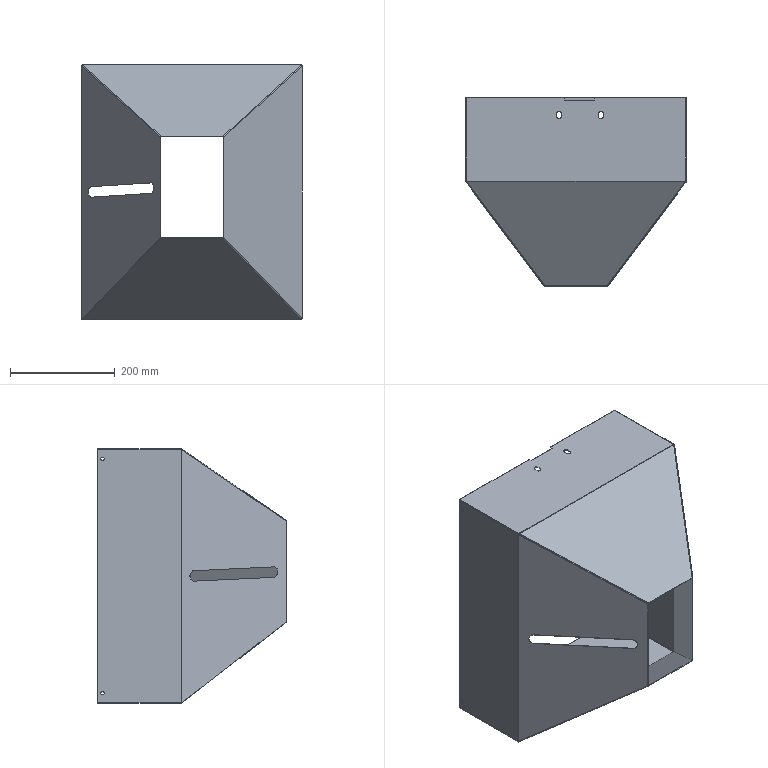Part | STEP file | JBJ-P-1001-01 | 2 solids | 88 faces | box 422 x 360.733 x 487 mm | volume 588476 mm3 | plane 56 | cylinder 26 | spline 6 | commonest cylinder face diameters 8.5 x8 2 x6 4 x6 6.5 x4 20 x2